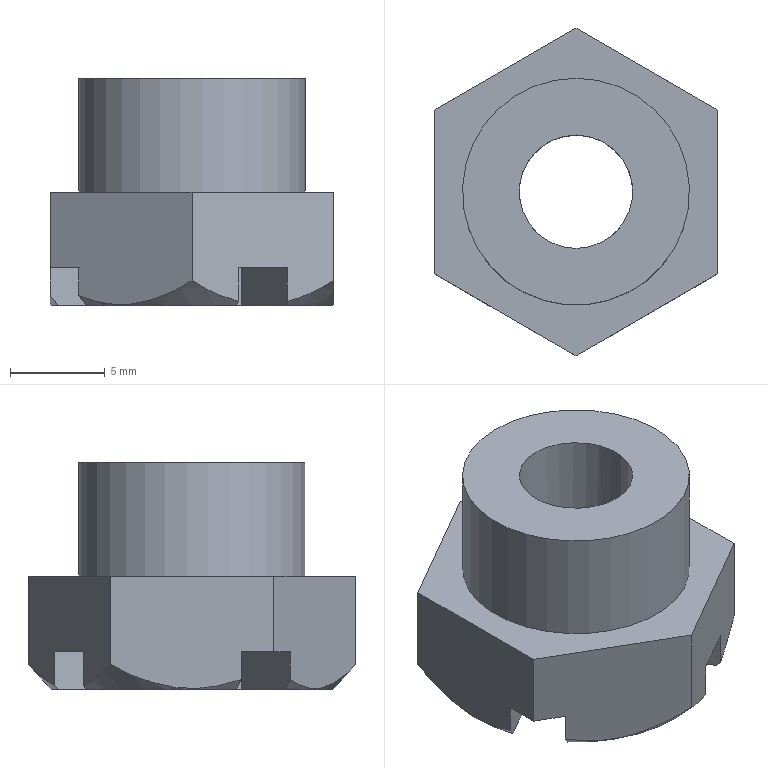Part | STEP file | 1-46.5 | 1 solid | 30 faces | box 15 x 17.321 x 12 mm | volume 1383 mm3 | plane 24 | cone 4 | cylinder 2 | commonest cylinder face diameters 6 x1 12 x1